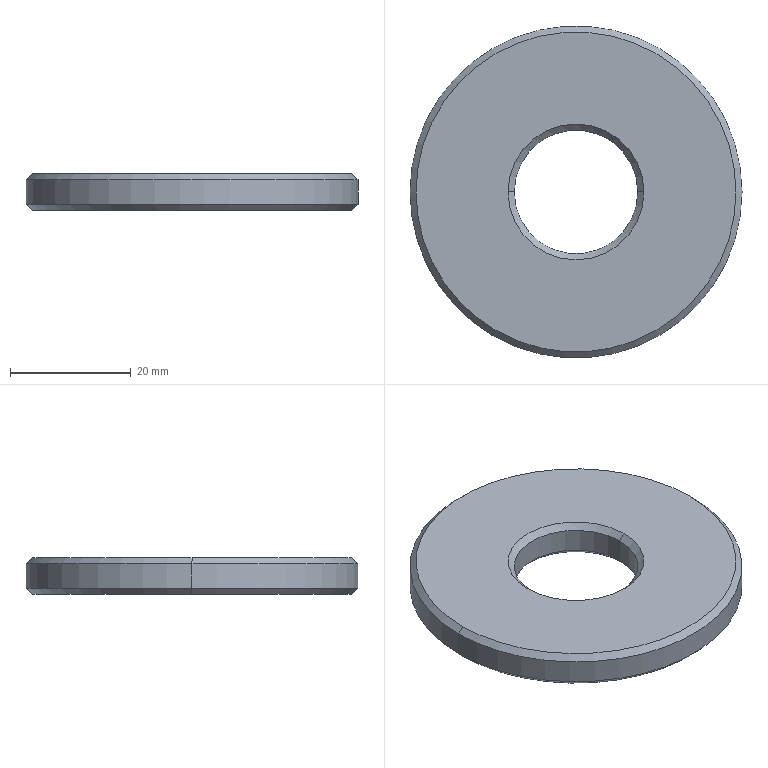Part | STEP file | YCD14007A-08.02.19A Lifting Cylinder Joint Stop Plate Added | 1 solid | 14 faces | box 55 x 55 x 6 mm | volume 12037 mm3 | cone 8 | cylinder 4 | plane 2 | commonest cylinder face diameters 20.5 x2 55 x2
STEP:
#1=CARTESIAN_POINT('',(0.,0.,0.));
#2=DIRECTION('',(0.,0.,1.));
#3=DIRECTION('',(1.,0.,0.));
#4=AXIS2_PLACEMENT_3D('',#1,#2,#3);
#5=CARTESIAN_POINT('',(-26.5,0.,-3.));
#6=VERTEX_POINT('',#5);
#7=CARTESIAN_POINT('',(26.5,0.,-3.));
#8=VERTEX_POINT('',#7);
#9=CARTESIAN_POINT('',(0.,0.,-3.));
#10=DIRECTION('',(0.,0.,-1.));
#11=DIRECTION('',(-1.,0.,0.));
#12=AXIS2_PLACEMENT_3D('',#9,#10,#11);
#13=CIRCLE('',#12,26.5);
#14=CARTESIAN_POINT('',(0.,0.,-2.));
#15=DIRECTION('',(0.,0.,1.));
#16=DIRECTION('',(1.,0.,0.));
#17=AXIS2_PLACEMENT_3D('',#14,#15,#16);
#18=CONICAL_SURFACE('',#17,27.5,0.7854);
#19=CARTESIAN_POINT('',(3.142,-1.));
#20=DIRECTION('',(-1.,0.));
#21=VECTOR('',#20,1.);
#22=LINE('',#19,#21);
#23=(GEOMETRIC_REPRESENTATION_CONTEXT(2)PARAMETRIC_REPRESENTATION_CONTEXT()REPRESENTATION_CONTEXT('',''));
#24=DEFINITIONAL_REPRESENTATION('',(#22),#23);
#25=PCURVE('',#18,#24);
#26=CARTESIAN_POINT('',(27.5,0.,-3.));
#27=DIRECTION('',(0.,0.,-1.));
#28=DIRECTION('',(-1.,0.,0.));
#29=AXIS2_PLACEMENT_3D('',#26,#27,#28);
#30=PLANE('',#29);
#31=CARTESIAN_POINT('',(27.5,0.));
#32=DIRECTION('',(1.,0.));
#33=AXIS2_PLACEMENT_2D('',#31,#32);
#34=CIRCLE('',#33,26.5);
#35=(GEOMETRIC_REPRESENTATION_CONTEXT(2)PARAMETRIC_REPRESENTATION_CONTEXT()REPRESENTATION_CONTEXT('',''));
#36=DEFINITIONAL_REPRESENTATION('',(#34),#35);
#37=PCURVE('',#30,#36);
#38=SURFACE_CURVE('',#13,(#25,#37),.PCURVE_S1.);
#39=EDGE_CURVE('',#6,#8,#38,.T.);
#40=ORIENTED_EDGE('',*,*,#39,.F.);
#41=CARTESIAN_POINT('',(-27.5,0.,-2.));
#42=VERTEX_POINT('',#41);
#43=CARTESIAN_POINT('',(-27.5,0.,-2.));
#44=DIRECTION('',(-0.7071,0.,0.7071));
#45=VECTOR('',#44,1.);
#46=LINE('',#43,#45);
#47=CARTESIAN_POINT('',(3.142,0.));
#48=DIRECTION('',(0.,1.));
#49=VECTOR('',#48,1.);
#50=LINE('',#47,#49);
#51=(GEOMETRIC_REPRESENTATION_CONTEXT(2)PARAMETRIC_REPRESENTATION_CONTEXT()REPRESENTATION_CONTEXT('',''));
#52=DEFINITIONAL_REPRESENTATION('',(#50),#51);
#53=PCURVE('',#18,#52);
#54=CARTESIAN_POINT('',(0.,0.,-2.));
#55=DIRECTION('',(0.,0.,1.));
#56=DIRECTION('',(1.,0.,0.));
#57=AXIS2_PLACEMENT_3D('',#54,#55,#56);
#58=CONICAL_SURFACE('',#57,27.5,0.7854);
#59=CARTESIAN_POINT('',(3.142,0.));
#60=DIRECTION('',(0.,1.));
#61=VECTOR('',#60,1.);
#62=LINE('',#59,#61);
#63=(GEOMETRIC_REPRESENTATION_CONTEXT(2)PARAMETRIC_REPRESENTATION_CONTEXT()REPRESENTATION_CONTEXT('',''));
#64=DEFINITIONAL_REPRESENTATION('',(#62),#63);
#65=PCURVE('',#58,#64);
#66=SURFACE_CURVE('',#46,(#53,#65),.PCURVE_S1.);
#67=EDGE_CURVE('',#6,#42,#66,.T.);
#68=ORIENTED_EDGE('',*,*,#67,.T.);
#69=CARTESIAN_POINT('',(27.5,0.,-2.));
#70=VERTEX_POINT('',#69);
#71=CARTESIAN_POINT('',(0.,0.,-2.));
#72=DIRECTION('',(0.,0.,1.));
#73=DIRECTION('',(-1.,0.,0.));
#74=AXIS2_PLACEMENT_3D('',#71,#72,#73);
#75=CIRCLE('',#74,27.5);
#76=CARTESIAN_POINT('',(-3.142,0.));
#77=DIRECTION('',(1.,0.));
#78=VECTOR('',#77,1.);
#79=LINE('',#76,#78);
#80=(GEOMETRIC_REPRESENTATION_CONTEXT(2)PARAMETRIC_REPRESENTATION_CONTEXT()REPRESENTATION_CONTEXT('',''));
#81=DEFINITIONAL_REPRESENTATION('',(#79),#80);
#82=PCURVE('',#18,#81);
#83=CARTESIAN_POINT('',(0.,0.,1000.));
#84=DIRECTION('',(0.,0.,1.));
#85=DIRECTION('',(1.,0.,0.));
#86=AXIS2_PLACEMENT_3D('',#83,#84,#85);
#87=CYLINDRICAL_SURFACE('',#86,27.5);
#88=CARTESIAN_POINT('',(-3.142,-1002.));
#89=DIRECTION('',(1.,0.));
#90=VECTOR('',#89,1.);
#91=LINE('',#88,#90);
#92=(GEOMETRIC_REPRESENTATION_CONTEXT(2)PARAMETRIC_REPRESENTATION_CONTEXT()REPRESENTATION_CONTEXT('',''));
#93=DEFINITIONAL_REPRESENTATION('',(#91),#92);
#94=PCURVE('',#87,#93);
#95=SURFACE_CURVE('',#75,(#82,#94),.PCURVE_S1.);
#96=EDGE_CURVE('',#70,#42,#95,.T.);
#97=ORIENTED_EDGE('',*,*,#96,.F.);
#98=CARTESIAN_POINT('',(27.5,0.,-2.));
#99=DIRECTION('',(0.7071,0.,0.7071));
#100=VECTOR('',#99,1.);
#101=LINE('',#98,#100);
#102=CARTESIAN_POINT('',(0.,0.));
#103=DIRECTION('',(0.,1.));
#104=VECTOR('',#103,1.);
#105=LINE('',#102,#104);
#106=(GEOMETRIC_REPRESENTATION_CONTEXT(2)PARAMETRIC_REPRESENTATION_CONTEXT()REPRESENTATION_CONTEXT('',''));
#107=DEFINITIONAL_REPRESENTATION('',(#105),#106);
#108=PCURVE('',#18,#107);
#109=CARTESIAN_POINT('',(6.283,0.));
#110=DIRECTION('',(0.,1.));
#111=VECTOR('',#110,1.);
#112=LINE('',#109,#111);
#113=(GEOMETRIC_REPRESENTATION_CONTEXT(2)PARAMETRIC_REPRESENTATION_CONTEXT()REPRESENTATION_CONTEXT('',''));
#114=DEFINITIONAL_REPRESENTATION('',(#112),#113);
#115=PCURVE('',#58,#114);
#116=SURFACE_CURVE('',#101,(#108,#115),.PCURVE_S1.);
#117=EDGE_CURVE('',#8,#70,#116,.T.);
#118=ORIENTED_EDGE('',*,*,#117,.F.);
#119=EDGE_LOOP('',(#40,#68,#97,#118));
#120=FACE_BOUND('',#119,.T.);
#121=ADVANCED_FACE('',(#120),#18,.T.);
#122=CARTESIAN_POINT('',(26.5,0.,3.));
#123=VERTEX_POINT('',#122);
#124=CARTESIAN_POINT('',(-26.5,0.,3.));
#125=VERTEX_POINT('',#124);
#126=CARTESIAN_POINT('',(0.,0.,3.));
#127=DIRECTION('',(0.,0.,1.));
#128=DIRECTION('',(1.,0.,0.));
#129=AXIS2_PLACEMENT_3D('',#126,#127,#128);
#130=CIRCLE('',#129,26.5);
#131=CARTESIAN_POINT('',(0.,0.,3.));
#132=DIRECTION('',(0.,0.,-1.));
#133=DIRECTION('',(-1.,0.,0.));
#134=AXIS2_PLACEMENT_3D('',#131,#132,#133);
#135=CONICAL_SURFACE('',#134,26.5,0.7854);
#136=CARTESIAN_POINT('',(3.142,0.));
#137=DIRECTION('',(-1.,0.));
#138=VECTOR('',#137,1.);
#139=LINE('',#136,#138);
#140=(GEOMETRIC_REPRESENTATION_CONTEXT(2)PARAMETRIC_REPRESENTATION_CONTEXT()REPRESENTATION_CONTEXT('',''));
#141=DEFINITIONAL_REPRESENTATION('',(#139),#140);
#142=PCURVE('',#135,#141);
#143=CARTESIAN_POINT('',(10.25,0.,3.));
#144=DIRECTION('',(0.,0.,1.));
#145=DIRECTION('',(1.,0.,0.));
#146=AXIS2_PLACEMENT_3D('',#143,#144,#145);
#147=PLANE('',#146);
#148=CARTESIAN_POINT('',(-10.25,0.));
#149=DIRECTION('',(1.,0.));
#150=AXIS2_PLACEMENT_2D('',#148,#149);
#151=CIRCLE('',#150,26.5);
#152=(GEOMETRIC_REPRESENTATION_CONTEXT(2)PARAMETRIC_REPRESENTATION_CONTEXT()REPRESENTATION_CONTEXT('',''));
#153=DEFINITIONAL_REPRESENTATION('',(#151),#152);
#154=PCURVE('',#147,#153);
#155=SURFACE_CURVE('',#130,(#142,#154),.PCURVE_S1.);
#156=EDGE_CURVE('',#123,#125,#155,.T.);
#157=ORIENTED_EDGE('',*,*,#156,.F.);
#158=CARTESIAN_POINT('',(27.5,0.,2.));
#159=VERTEX_POINT('',#158);
#160=CARTESIAN_POINT('',(26.5,0.,3.));
#161=DIRECTION('',(0.7071,0.,-0.7071));
#162=VECTOR('',#161,1.);
#163=LINE('',#160,#162);
#164=CARTESIAN_POINT('',(3.142,0.));
#165=DIRECTION('',(0.,1.));
#166=VECTOR('',#165,1.);
#167=LINE('',#164,#166);
#168=(GEOMETRIC_REPRESENTATION_CONTEXT(2)PARAMETRIC_REPRESENTATION_CONTEXT()REPRESENTATION_CONTEXT('',''));
#169=DEFINITIONAL_REPRESENTATION('',(#167),#168);
#170=PCURVE('',#135,#169);
#171=CARTESIAN_POINT('',(0.,0.,3.));
#172=DIRECTION('',(0.,0.,-1.));
#173=DIRECTION('',(-1.,0.,0.));
#174=AXIS2_PLACEMENT_3D('',#171,#172,#173);
#175=CONICAL_SURFACE('',#174,26.5,0.7854);
#176=CARTESIAN_POINT('',(3.142,0.));
#177=DIRECTION('',(0.,1.));
#178=VECTOR('',#177,1.);
#179=LINE('',#176,#178);
#180=(GEOMETRIC_REPRESENTATION_CONTEXT(2)PARAMETRIC_REPRESENTATION_CONTEXT()REPRESENTATION_CONTEXT('',''));
#181=DEFINITIONAL_REPRESENTATION('',(#179),#180);
#182=PCURVE('',#175,#181);
#183=SURFACE_CURVE('',#163,(#170,#182),.PCURVE_S1.);
#184=EDGE_CURVE('',#123,#159,#183,.T.);
#185=ORIENTED_EDGE('',*,*,#184,.T.);
#186=CARTESIAN_POINT('',(-27.5,0.,2.));
#187=VERTEX_POINT('',#186);
#188=CARTESIAN_POINT('',(0.,0.,2.));
#189=DIRECTION('',(0.,0.,-1.));
#190=DIRECTION('',(1.,0.,0.));
#191=AXIS2_PLACEMENT_3D('',#188,#189,#190);
#192=CIRCLE('',#191,27.5);
#193=CARTESIAN_POINT('',(-3.142,1.));
#194=DIRECTION('',(1.,0.));
#195=VECTOR('',#194,1.);
#196=LINE('',#193,#195);
#197=(GEOMETRIC_REPRESENTATION_CONTEXT(2)PARAMETRIC_REPRESENTATION_CONTEXT()REPRESENTATION_CONTEXT('',''));
#198=DEFINITIONAL_REPRESENTATION('',(#196),#197);
#199=PCURVE('',#135,#198);
#200=CARTESIAN_POINT('',(6.283,-998.));
#201=DIRECTION('',(-1.,0.));
#202=VECTOR('',#201,1.);
#203=LINE('',#200,#202);
#204=(GEOMETRIC_REPRESENTATION_CONTEXT(2)PARAMETRIC_REPRESENTATION_CONTEXT()REPRESENTATION_CONTEXT('',''));
#205=DEFINITIONAL_REPRESENTATION('',(#203),#204);
#206=PCURVE('',#87,#205);
#207=SURFACE_CURVE('',#192,(#199,#206),.PCURVE_S1.);
#208=EDGE_CURVE('',#187,#159,#207,.T.);
#209=ORIENTED_EDGE('',*,*,#208,.F.);
#210=CARTESIAN_POINT('',(-26.5,0.,3.));
#211=DIRECTION('',(-0.7071,0.,-0.7071));
#212=VECTOR('',#211,1.);
#213=LINE('',#210,#212);
#214=CARTESIAN_POINT('',(0.,0.));
#215=DIRECTION('',(0.,1.));
#216=VECTOR('',#215,1.);
#217=LINE('',#214,#216);
#218=(GEOMETRIC_REPRESENTATION_CONTEXT(2)PARAMETRIC_REPRESENTATION_CONTEXT()REPRESENTATION_CONTEXT('',''));
#219=DEFINITIONAL_REPRESENTATION('',(#217),#218);
#220=PCURVE('',#135,#219);
#221=CARTESIAN_POINT('',(6.283,0.));
#222=DIRECTION('',(0.,1.));
#223=VECTOR('',#222,1.);
#224=LINE('',#221,#223);
#225=(GEOMETRIC_REPRESENTATION_CONTEXT(2)PARAMETRIC_REPRESENTATION_CONTEXT()REPRESENTATION_CONTEXT('',''));
#226=DEFINITIONAL_REPRESENTATION('',(#224),#225);
#227=PCURVE('',#175,#226);
#228=SURFACE_CURVE('',#213,(#220,#227),.PCURVE_S1.);
#229=EDGE_CURVE('',#125,#187,#228,.T.);
#230=ORIENTED_EDGE('',*,*,#229,.F.);
#231=EDGE_LOOP('',(#157,#185,#209,#230));
#232=FACE_BOUND('',#231,.T.);
#233=ADVANCED_FACE('',(#232),#135,.T.);
#234=CARTESIAN_POINT('',(-10.25,0.,-2.));
#235=VERTEX_POINT('',#234);
#236=CARTESIAN_POINT('',(-11.25,0.,-3.));
#237=VERTEX_POINT('',#236);
#238=CARTESIAN_POINT('',(-11.25,0.,-3.));
#239=DIRECTION('',(-0.7071,0.,-0.7071));
#240=VECTOR('',#239,1.);
#241=LINE('',#238,#240);
#242=CARTESIAN_POINT('',(0.,0.,-3.));
#243=DIRECTION('',(0.,0.,-1.));
#244=DIRECTION('',(-1.,0.,0.));
#245=AXIS2_PLACEMENT_3D('',#242,#243,#244);
#246=CONICAL_SURFACE('',#245,11.25,0.7854);
#247=CARTESIAN_POINT('',(6.283,0.));
#248=DIRECTION('',(0.,1.));
#249=VECTOR('',#248,1.);
#250=LINE('',#247,#249);
#251=(GEOMETRIC_REPRESENTATION_CONTEXT(2)PARAMETRIC_REPRESENTATION_CONTEXT()REPRESENTATION_CONTEXT('',''));
#252=DEFINITIONAL_REPRESENTATION('',(#250),#251);
#253=PCURVE('',#246,#252);
#254=CARTESIAN_POINT('',(0.,0.,-3.));
#255=DIRECTION('',(0.,0.,-1.));
#256=DIRECTION('',(-1.,0.,0.));
#257=AXIS2_PLACEMENT_3D('',#254,#255,#256);
#258=CONICAL_SURFACE('',#257,11.25,0.7854);
#259=CARTESIAN_POINT('',(0.,0.));
#260=DIRECTION('',(0.,1.));
#261=VECTOR('',#260,1.);
#262=LINE('',#259,#261);
#263=(GEOMETRIC_REPRESENTATION_CONTEXT(2)PARAMETRIC_REPRESENTATION_CONTEXT()REPRESENTATION_CONTEXT('',''));
#264=DEFINITIONAL_REPRESENTATION('',(#262),#263);
#265=PCURVE('',#258,#264);
#266=SURFACE_CURVE('',#241,(#253,#265),.PCURVE_S1.);
#267=EDGE_CURVE('',#235,#237,#266,.T.);
#268=ORIENTED_EDGE('',*,*,#267,.T.);
#269=CARTESIAN_POINT('',(11.25,0.,-3.));
#270=VERTEX_POINT('',#269);
#271=CARTESIAN_POINT('',(0.,0.,-3.));
#272=DIRECTION('',(0.,0.,1.));
#273=DIRECTION('',(-1.,0.,0.));
#274=AXIS2_PLACEMENT_3D('',#271,#272,#273);
#275=CIRCLE('',#274,11.25);
#276=CARTESIAN_POINT('',(6.283,0.));
#277=DIRECTION('',(-1.,0.));
#278=VECTOR('',#277,1.);
#279=LINE('',#276,#278);
#280=(GEOMETRIC_REPRESENTATION_CONTEXT(2)PARAMETRIC_REPRESENTATION_CONTEXT()REPRESENTATION_CONTEXT('',''));
#281=DEFINITIONAL_REPRESENTATION('',(#279),#280);
#282=PCURVE('',#246,#281);
#283=CARTESIAN_POINT('',(38.75,0.));
#284=CARTESIAN_POINT('',(38.75,-19.486));
#285=CARTESIAN_POINT('',(21.875,-9.743));
#286=CARTESIAN_POINT('',(5.,0.));
#287=CARTESIAN_POINT('',(21.875,9.743));
#288=CARTESIAN_POINT('',(38.75,19.486));
#289=CARTESIAN_POINT('',(38.75,0.));
#290=(BOUNDED_CURVE()B_SPLINE_CURVE(2,(#283,#284,#285,#286,#287,#288,#289),.UNSPECIFIED.,.T.,.F.)B_SPLINE_CURVE_WITH_KNOTS((1,2,2,2,2,1),(-2.094,0.,2.094,4.189,6.283,8.378),.UNSPECIFIED.)CURVE()GEOMETRIC_REPRESENTATION_ITEM()RATIONAL_B_SPLINE_CURVE((1.,0.5,1.,0.5,1.,0.5,1.))REPRESENTATION_ITEM(''));
#291=(GEOMETRIC_REPRESENTATION_CONTEXT(2)PARAMETRIC_REPRESENTATION_CONTEXT()REPRESENTATION_CONTEXT('',''));
#292=DEFINITIONAL_REPRESENTATION('',(#290),#291);
#293=PCURVE('',#30,#292);
#294=SURFACE_CURVE('',#275,(#282,#293),.PCURVE_S1.);
#295=EDGE_CURVE('',#237,#270,#294,.T.);
#296=ORIENTED_EDGE('',*,*,#295,.T.);
#297=CARTESIAN_POINT('',(10.25,0.,-2.));
#298=VERTEX_POINT('',#297);
#299=CARTESIAN_POINT('',(11.25,0.,-3.));
#300=DIRECTION('',(0.7071,0.,-0.7071));
#301=VECTOR('',#300,1.);
#302=LINE('',#299,#301);
#303=CARTESIAN_POINT('',(3.142,0.));
#304=DIRECTION('',(0.,1.));
#305=VECTOR('',#304,1.);
#306=LINE('',#303,#305);
#307=(GEOMETRIC_REPRESENTATION_CONTEXT(2)PARAMETRIC_REPRESENTATION_CONTEXT()REPRESENTATION_CONTEXT('',''));
#308=DEFINITIONAL_REPRESENTATION('',(#306),#307);
#309=PCURVE('',#246,#308);
#310=CARTESIAN_POINT('',(3.142,0.));
#311=DIRECTION('',(0.,1.));
#312=VECTOR('',#311,1.);
#313=LINE('',#310,#312);
#314=(GEOMETRIC_REPRESENTATION_CONTEXT(2)PARAMETRIC_REPRESENTATION_CONTEXT()REPRESENTATION_CONTEXT('',''));
#315=DEFINITIONAL_REPRESENTATION('',(#313),#314);
#316=PCURVE('',#258,#315);
#317=SURFACE_CURVE('',#302,(#309,#316),.PCURVE_S1.);
#318=EDGE_CURVE('',#298,#270,#317,.T.);
#319=ORIENTED_EDGE('',*,*,#318,.F.);
#320=CARTESIAN_POINT('',(0.,0.,-2.));
#321=DIRECTION('',(0.,0.,-1.));
#322=DIRECTION('',(-1.,0.,0.));
#323=AXIS2_PLACEMENT_3D('',#320,#321,#322);
#324=CIRCLE('',#323,10.25);
#325=CARTESIAN_POINT('',(0.,-1.));
#326=DIRECTION('',(1.,0.));
#327=VECTOR('',#326,1.);
#328=LINE('',#325,#327);
#329=(GEOMETRIC_REPRESENTATION_CONTEXT(2)PARAMETRIC_REPRESENTATION_CONTEXT()REPRESENTATION_CONTEXT('',''));
#330=DEFINITIONAL_REPRESENTATION('',(#328),#329);
#331=PCURVE('',#246,#330);
#332=CARTESIAN_POINT('',(0.,0.,1000.));
#333=DIRECTION('',(0.,0.,1.));
#334=DIRECTION('',(1.,0.,0.));
#335=AXIS2_PLACEMENT_3D('',#332,#333,#334);
#336=CYLINDRICAL_SURFACE('',#335,10.25);
#337=CARTESIAN_POINT('',(9.425,-1002.));
#338=DIRECTION('',(-1.,0.));
#339=VECTOR('',#338,1.);
#340=LINE('',#337,#339);
#341=(GEOMETRIC_REPRESENTATION_CONTEXT(2)PARAMETRIC_REPRESENTATION_CONTEXT()REPRESENTATION_CONTEXT('',''));
#342=DEFINITIONAL_REPRESENTATION('',(#340),#341);
#343=PCURVE('',#336,#342);
#344=SURFACE_CURVE('',#324,(#331,#343),.PCURVE_S1.);
#345=EDGE_CURVE('',#298,#235,#344,.T.);
#346=ORIENTED_EDGE('',*,*,#345,.T.);
#347=EDGE_LOOP('',(#268,#296,#319,#346));
#348=FACE_BOUND('',#347,.F.);
#349=ADVANCED_FACE('',(#348),#246,.F.);
#350=CARTESIAN_POINT('',(10.25,0.,2.));
#351=VERTEX_POINT('',#350);
#352=CARTESIAN_POINT('',(11.25,0.,3.));
#353=VERTEX_POINT('',#352);
#354=CARTESIAN_POINT('',(10.25,0.,2.));
#355=DIRECTION('',(0.7071,0.,0.7071));
#356=VECTOR('',#355,1.);
#357=LINE('',#354,#356);
#358=CARTESIAN_POINT('',(0.,0.,2.));
#359=DIRECTION('',(0.,0.,1.));
#360=DIRECTION('',(1.,0.,0.));
#361=AXIS2_PLACEMENT_3D('',#358,#359,#360);
#362=CONICAL_SURFACE('',#361,10.25,0.7854);
#363=CARTESIAN_POINT('',(6.283,0.));
#364=DIRECTION('',(0.,1.));
#365=VECTOR('',#364,1.);
#366=LINE('',#363,#365);
#367=(GEOMETRIC_REPRESENTATION_CONTEXT(2)PARAMETRIC_REPRESENTATION_CONTEXT()REPRESENTATION_CONTEXT('',''));
#368=DEFINITIONAL_REPRESENTATION('',(#366),#367);
#369=PCURVE('',#362,#368);
#370=CARTESIAN_POINT('',(0.,0.,2.));
#371=DIRECTION('',(0.,0.,1.));
#372=DIRECTION('',(1.,0.,0.));
#373=AXIS2_PLACEMENT_3D('',#370,#371,#372);
#374=CONICAL_SURFACE('',#373,10.25,0.7854);
#375=CARTESIAN_POINT('',(0.,0.));
#376=DIRECTION('',(0.,1.));
#377=VECTOR('',#376,1.);
#378=LINE('',#375,#377);
#379=(GEOMETRIC_REPRESENTATION_CONTEXT(2)PARAMETRIC_REPRESENTATION_CONTEXT()REPRESENTATION_CONTEXT('',''));
#380=DEFINITIONAL_REPRESENTATION('',(#378),#379);
#381=PCURVE('',#374,#380);
#382=SURFACE_CURVE('',#357,(#369,#381),.PCURVE_S1.);
#383=EDGE_CURVE('',#351,#353,#382,.T.);
#384=ORIENTED_EDGE('',*,*,#383,.T.);
#385=CARTESIAN_POINT('',(-11.25,0.,3.));
#386=VERTEX_POINT('',#385);
#387=CARTESIAN_POINT('',(0.,0.,3.));
#388=DIRECTION('',(0.,0.,-1.));
#389=DIRECTION('',(1.,0.,0.));
#390=AXIS2_PLACEMENT_3D('',#387,#388,#389);
#391=CIRCLE('',#390,11.25);
#392=CARTESIAN_POINT('',(6.283,1.));
#393=DIRECTION('',(-1.,0.));
#394=VECTOR('',#393,1.);
#395=LINE('',#392,#394);
#396=(GEOMETRIC_REPRESENTATION_CONTEXT(2)PARAMETRIC_REPRESENTATION_CONTEXT()REPRESENTATION_CONTEXT('',''));
#397=DEFINITIONAL_REPRESENTATION('',(#395),#396);
#398=PCURVE('',#362,#397);
#399=CARTESIAN_POINT('',(1.,0.));
#400=CARTESIAN_POINT('',(1.,-19.486));
#401=CARTESIAN_POINT('',(-15.875,-9.743));
#402=CARTESIAN_POINT('',(-32.75,0.));
#403=CARTESIAN_POINT('',(-15.875,9.743));
#404=CARTESIAN_POINT('',(1.,19.486));
#405=CARTESIAN_POINT('',(1.,0.));
#406=(BOUNDED_CURVE()B_SPLINE_CURVE(2,(#399,#400,#401,#402,#403,#404,#405),.UNSPECIFIED.,.T.,.F.)B_SPLINE_CURVE_WITH_KNOTS((1,2,2,2,2,1),(-2.094,0.,2.094,4.189,6.283,8.378),.UNSPECIFIED.)CURVE()GEOMETRIC_REPRESENTATION_ITEM()RATIONAL_B_SPLINE_CURVE((1.,0.5,1.,0.5,1.,0.5,1.))REPRESENTATION_ITEM(''));
#407=(GEOMETRIC_REPRESENTATION_CONTEXT(2)PARAMETRIC_REPRESENTATION_CONTEXT()REPRESENTATION_CONTEXT('',''));
#408=DEFINITIONAL_REPRESENTATION('',(#406),#407);
#409=PCURVE('',#147,#408);
#410=SURFACE_CURVE('',#391,(#398,#409),.PCURVE_S1.);
#411=EDGE_CURVE('',#353,#386,#410,.T.);
#412=ORIENTED_EDGE('',*,*,#411,.T.);
#413=CARTESIAN_POINT('',(-10.25,0.,2.));
#414=VERTEX_POINT('',#413);
#415=CARTESIAN_POINT('',(-10.25,0.,2.));
#416=DIRECTION('',(-0.7071,0.,0.7071));
#417=VECTOR('',#416,1.);
#418=LINE('',#415,#417);
#419=CARTESIAN_POINT('',(3.142,0.));
#420=DIRECTION('',(0.,1.));
#421=VECTOR('',#420,1.);
#422=LINE('',#419,#421);
#423=(GEOMETRIC_REPRESENTATION_CONTEXT(2)PARAMETRIC_REPRESENTATION_CONTEXT()REPRESENTATION_CONTEXT('',''));
#424=DEFINITIONAL_REPRESENTATION('',(#422),#423);
#425=PCURVE('',#362,#424);
#426=CARTESIAN_POINT('',(3.142,0.));
#427=DIRECTION('',(0.,1.));
#428=VECTOR('',#427,1.);
#429=LINE('',#426,#428);
#430=(GEOMETRIC_REPRESENTATION_CONTEXT(2)PARAMETRIC_REPRESENTATION_CONTEXT()REPRESENTATION_CONTEXT('',''));
#431=DEFINITIONAL_REPRESENTATION('',(#429),#430);
#432=PCURVE('',#374,#431);
#433=SURFACE_CURVE('',#418,(#425,#432),.PCURVE_S1.);
#434=EDGE_CURVE('',#414,#386,#433,.T.);
#435=ORIENTED_EDGE('',*,*,#434,.F.);
#436=CARTESIAN_POINT('',(0.,0.,2.));
#437=DIRECTION('',(0.,0.,1.));
#438=DIRECTION('',(1.,0.,0.));
#439=AXIS2_PLACEMENT_3D('',#436,#437,#438);
#440=CIRCLE('',#439,10.25);
#441=CARTESIAN_POINT('',(0.,0.));
#442=DIRECTION('',(1.,0.));
#443=VECTOR('',#442,1.);
#444=LINE('',#441,#443);
#445=(GEOMETRIC_REPRESENTATION_CONTEXT(2)PARAMETRIC_REPRESENTATION_CONTEXT()REPRESENTATION_CONTEXT('',''));
#446=DEFINITIONAL_REPRESENTATION('',(#444),#445);
#447=PCURVE('',#362,#446);
#448=CARTESIAN_POINT('',(0.,-998.));
#449=DIRECTION('',(1.,0.));
#450=VECTOR('',#449,1.);
#451=LINE('',#448,#450);
#452=(GEOMETRIC_REPRESENTATION_CONTEXT(2)PARAMETRIC_REPRESENTATION_CONTEXT()REPRESENTATION_CONTEXT('',''));
#453=DEFINITIONAL_REPRESENTATION('',(#451),#452);
#454=PCURVE('',#336,#453);
#455=SURFACE_CURVE('',#440,(#447,#454),.PCURVE_S1.);
#456=EDGE_CURVE('',#414,#351,#455,.T.);
#457=ORIENTED_EDGE('',*,*,#456,.T.);
#458=EDGE_LOOP('',(#384,#412,#435,#457));
#459=FACE_BOUND('',#458,.F.);
#460=ADVANCED_FACE('',(#459),#362,.F.);
#461=CARTESIAN_POINT('',(10.25,0.,1000.));
#462=DIRECTION('',(0.,0.,1.));
#463=VECTOR('',#462,1.);
#464=LINE('',#461,#463);
#465=CARTESIAN_POINT('',(6.283,0.));
#466=DIRECTION('',(0.,1.));
#467=VECTOR('',#466,1.);
#468=LINE('',#465,#467);
#469=(GEOMETRIC_REPRESENTATION_CONTEXT(2)PARAMETRIC_REPRESENTATION_CONTEXT()REPRESENTATION_CONTEXT('',''));
#470=DEFINITIONAL_REPRESENTATION('',(#468),#469);
#471=PCURVE('',#336,#470);
#472=CARTESIAN_POINT('',(0.,0.,1000.));
#473=DIRECTION('',(0.,0.,1.));
#474=DIRECTION('',(1.,0.,0.));
#475=AXIS2_PLACEMENT_3D('',#472,#473,#474);
#476=CYLINDRICAL_SURFACE('',#475,10.25);
#477=CARTESIAN_POINT('',(0.,0.));
#478=DIRECTION('',(0.,1.));
#479=VECTOR('',#478,1.);
#480=LINE('',#477,#479);
#481=(GEOMETRIC_REPRESENTATION_CONTEXT(2)PARAMETRIC_REPRESENTATION_CONTEXT()REPRESENTATION_CONTEXT('',''));
#482=DEFINITIONAL_REPRESENTATION('',(#480),#481);
#483=PCURVE('',#476,#482);
#484=SURFACE_CURVE('',#464,(#471,#483),.PCURVE_S1.);
#485=EDGE_CURVE('',#298,#351,#484,.T.);
#486=ORIENTED_EDGE('',*,*,#485,.T.);
#487=ORIENTED_EDGE('',*,*,#456,.F.);
#488=CARTESIAN_POINT('',(-10.25,0.,1000.));
#489=DIRECTION('',(0.,0.,1.));
#490=VECTOR('',#489,1.);
#491=LINE('',#488,#490);
#492=CARTESIAN_POINT('',(3.142,0.));
#493=DIRECTION('',(0.,1.));
#494=VECTOR('',#493,1.);
#495=LINE('',#492,#494);
#496=(GEOMETRIC_REPRESENTATION_CONTEXT(2)PARAMETRIC_REPRESENTATION_CONTEXT()REPRESENTATION_CONTEXT('',''));
#497=DEFINITIONAL_REPRESENTATION('',(#495),#496);
#498=PCURVE('',#336,#497);
#499=CARTESIAN_POINT('',(3.142,0.));
#500=DIRECTION('',(0.,1.));
#501=VECTOR('',#500,1.);
#502=LINE('',#499,#501);
#503=(GEOMETRIC_REPRESENTATION_CONTEXT(2)PARAMETRIC_REPRESENTATION_CONTEXT()REPRESENTATION_CONTEXT('',''));
#504=DEFINITIONAL_REPRESENTATION('',(#502),#503);
#505=PCURVE('',#476,#504);
#506=SURFACE_CURVE('',#491,(#498,#505),.PCURVE_S1.);
#507=EDGE_CURVE('',#235,#414,#506,.T.);
#508=ORIENTED_EDGE('',*,*,#507,.F.);
#509=ORIENTED_EDGE('',*,*,#345,.F.);
#510=EDGE_LOOP('',(#486,#487,#508,#509));
#511=FACE_BOUND('',#510,.F.);
#512=ADVANCED_FACE('',(#511),#336,.F.);
#513=ORIENTED_EDGE('',*,*,#96,.T.);
#514=CARTESIAN_POINT('',(-27.5,0.,1000.));
#515=DIRECTION('',(0.,0.,1.));
#516=VECTOR('',#515,1.);
#517=LINE('',#514,#516);
#518=CARTESIAN_POINT('',(3.142,0.));
#519=DIRECTION('',(0.,1.));
#520=VECTOR('',#519,1.);
#521=LINE('',#518,#520);
#522=(GEOMETRIC_REPRESENTATION_CONTEXT(2)PARAMETRIC_REPRESENTATION_CONTEXT()REPRESENTATION_CONTEXT('',''));
#523=DEFINITIONAL_REPRESENTATION('',(#521),#522);
#524=PCURVE('',#87,#523);
#525=CARTESIAN_POINT('',(0.,0.,1000.));
#526=DIRECTION('',(0.,0.,1.));
#527=DIRECTION('',(1.,0.,0.));
#528=AXIS2_PLACEMENT_3D('',#525,#526,#527);
#529=CYLINDRICAL_SURFACE('',#528,27.5);
#530=CARTESIAN_POINT('',(3.142,0.));
#531=DIRECTION('',(0.,1.));
#532=VECTOR('',#531,1.);
#533=LINE('',#530,#532);
#534=(GEOMETRIC_REPRESENTATION_CONTEXT(2)PARAMETRIC_REPRESENTATION_CONTEXT()REPRESENTATION_CONTEXT('',''));
#535=DEFINITIONAL_REPRESENTATION('',(#533),#534);
#536=PCURVE('',#529,#535);
#537=SURFACE_CURVE('',#517,(#524,#536),.PCURVE_S1.);
#538=EDGE_CURVE('',#42,#187,#537,.T.);
#539=ORIENTED_EDGE('',*,*,#538,.T.);
#540=ORIENTED_EDGE('',*,*,#208,.T.);
#541=CARTESIAN_POINT('',(27.5,0.,1000.));
#542=DIRECTION('',(0.,0.,1.));
#543=VECTOR('',#542,1.);
#544=LINE('',#541,#543);
#545=CARTESIAN_POINT('',(0.,0.));
#546=DIRECTION('',(0.,1.));
#547=VECTOR('',#546,1.);
#548=LINE('',#545,#547);
#549=(GEOMETRIC_REPRESENTATION_CONTEXT(2)PARAMETRIC_REPRESENTATION_CONTEXT()REPRESENTATION_CONTEXT('',''));
#550=DEFINITIONAL_REPRESENTATION('',(#548),#549);
#551=PCURVE('',#87,#550);
#552=CARTESIAN_POINT('',(6.283,0.));
#553=DIRECTION('',(0.,1.));
#554=VECTOR('',#553,1.);
#555=LINE('',#552,#554);
#556=(GEOMETRIC_REPRESENTATION_CONTEXT(2)PARAMETRIC_REPRESENTATION_CONTEXT()REPRESENTATION_CONTEXT('',''));
#557=DEFINITIONAL_REPRESENTATION('',(#555),#556);
#558=PCURVE('',#529,#557);
#559=SURFACE_CURVE('',#544,(#551,#558),.PCURVE_S1.);
#560=EDGE_CURVE('',#70,#159,#559,.T.);
#561=ORIENTED_EDGE('',*,*,#560,.F.);
#562=EDGE_LOOP('',(#513,#539,#540,#561));
#563=FACE_BOUND('',#562,.T.);
#564=ADVANCED_FACE('',(#563),#87,.T.);
#565=ORIENTED_EDGE('',*,*,#538,.F.);
#566=CARTESIAN_POINT('',(0.,0.,-2.));
#567=DIRECTION('',(0.,0.,1.));
#568=DIRECTION('',(-1.,0.,0.));
#569=AXIS2_PLACEMENT_3D('',#566,#567,#568);
#570=CIRCLE('',#569,27.5);
#571=CARTESIAN_POINT('',(3.142,-1002.));
#572=DIRECTION('',(1.,0.));
#573=VECTOR('',#572,1.);
#574=LINE('',#571,#573);
#575=(GEOMETRIC_REPRESENTATION_CONTEXT(2)PARAMETRIC_REPRESENTATION_CONTEXT()REPRESENTATION_CONTEXT('',''));
#576=DEFINITIONAL_REPRESENTATION('',(#574),#575);
#577=PCURVE('',#529,#576);
#578=CARTESIAN_POINT('',(3.142,0.));
#579=DIRECTION('',(1.,0.));
#580=VECTOR('',#579,1.);
#581=LINE('',#578,#580);
#582=(GEOMETRIC_REPRESENTATION_CONTEXT(2)PARAMETRIC_REPRESENTATION_CONTEXT()REPRESENTATION_CONTEXT('',''));
#583=DEFINITIONAL_REPRESENTATION('',(#581),#582);
#584=PCURVE('',#58,#583);
#585=SURFACE_CURVE('',#570,(#577,#584),.PCURVE_S1.);
#586=EDGE_CURVE('',#42,#70,#585,.T.);
#587=ORIENTED_EDGE('',*,*,#586,.T.);
#588=ORIENTED_EDGE('',*,*,#560,.T.);
#589=CARTESIAN_POINT('',(0.,0.,2.));
#590=DIRECTION('',(0.,0.,-1.));
#591=DIRECTION('',(1.,0.,0.));
#592=AXIS2_PLACEMENT_3D('',#589,#590,#591);
#593=CIRCLE('',#592,27.5);
#594=CARTESIAN_POINT('',(6.283,-998.));
#595=DIRECTION('',(-1.,0.));
#596=VECTOR('',#595,1.);
#597=LINE('',#594,#596);
#598=(GEOMETRIC_REPRESENTATION_CONTEXT(2)PARAMETRIC_REPRESENTATION_CONTEXT()REPRESENTATION_CONTEXT('',''));
#599=DEFINITIONAL_REPRESENTATION('',(#597),#598);
#600=PCURVE('',#529,#599);
#601=CARTESIAN_POINT('',(3.142,1.));
#602=DIRECTION('',(1.,0.));
#603=VECTOR('',#602,1.);
#604=LINE('',#601,#603);
#605=(GEOMETRIC_REPRESENTATION_CONTEXT(2)PARAMETRIC_REPRESENTATION_CONTEXT()REPRESENTATION_CONTEXT('',''));
#606=DEFINITIONAL_REPRESENTATION('',(#604),#605);
#607=PCURVE('',#175,#606);
#608=SURFACE_CURVE('',#593,(#600,#607),.PCURVE_S1.);
#609=EDGE_CURVE('',#159,#187,#608,.T.);
#610=ORIENTED_EDGE('',*,*,#609,.T.);
#611=EDGE_LOOP('',(#565,#587,#588,#610));
#612=FACE_BOUND('',#611,.T.);
#613=ADVANCED_FACE('',(#612),#529,.T.);
#614=ORIENTED_EDGE('',*,*,#295,.T.);
#615=CARTESIAN_POINT('',(0.,0.,-3.));
#616=DIRECTION('',(0.,0.,1.));
#617=DIRECTION('',(-1.,0.,0.));
#618=AXIS2_PLACEMENT_3D('',#615,#616,#617);
#619=CIRCLE('',#618,11.25);
#620=CARTESIAN_POINT('',(38.75,0.));
#621=CARTESIAN_POINT('',(38.75,-19.486));
#622=CARTESIAN_POINT('',(21.875,-9.743));
#623=CARTESIAN_POINT('',(5.,0.));
#624=CARTESIAN_POINT('',(21.875,9.743));
#625=CARTESIAN_POINT('',(38.75,19.486));
#626=CARTESIAN_POINT('',(38.75,0.));
#627=(BOUNDED_CURVE()B_SPLINE_CURVE(2,(#620,#621,#622,#623,#624,#625,#626),.UNSPECIFIED.,.T.,.F.)B_SPLINE_CURVE_WITH_KNOTS((1,2,2,2,2,1),(-2.094,0.,2.094,4.189,6.283,8.378),.UNSPECIFIED.)CURVE()GEOMETRIC_REPRESENTATION_ITEM()RATIONAL_B_SPLINE_CURVE((1.,0.5,1.,0.5,1.,0.5,1.))REPRESENTATION_ITEM(''));
#628=(GEOMETRIC_REPRESENTATION_CONTEXT(2)PARAMETRIC_REPRESENTATION_CONTEXT()REPRESENTATION_CONTEXT('',''));
#629=DEFINITIONAL_REPRESENTATION('',(#627),#628);
#630=PCURVE('',#30,#629);
#631=CARTESIAN_POINT('',(6.283,0.));
#632=DIRECTION('',(-1.,0.));
#633=VECTOR('',#632,1.);
#634=LINE('',#631,#633);
#635=(GEOMETRIC_REPRESENTATION_CONTEXT(2)PARAMETRIC_REPRESENTATION_CONTEXT()REPRESENTATION_CONTEXT('',''));
#636=DEFINITIONAL_REPRESENTATION('',(#634),#635);
#637=PCURVE('',#258,#636);
#638=SURFACE_CURVE('',#619,(#630,#637),.PCURVE_S1.);
#639=EDGE_CURVE('',#270,#237,#638,.T.);
#640=ORIENTED_EDGE('',*,*,#639,.T.);
#641=EDGE_LOOP('',(#614,#640));
#642=FACE_BOUND('',#641,.T.);
#643=CARTESIAN_POINT('',(0.,0.,-3.));
#644=DIRECTION('',(0.,0.,-1.));
#645=DIRECTION('',(-1.,0.,0.));
#646=AXIS2_PLACEMENT_3D('',#643,#644,#645);
#647=CIRCLE('',#646,26.5);
#648=CARTESIAN_POINT('',(27.5,0.));
#649=DIRECTION('',(1.,0.));
#650=AXIS2_PLACEMENT_2D('',#648,#649);
#651=CIRCLE('',#650,26.5);
#652=(GEOMETRIC_REPRESENTATION_CONTEXT(2)PARAMETRIC_REPRESENTATION_CONTEXT()REPRESENTATION_CONTEXT('',''));
#653=DEFINITIONAL_REPRESENTATION('',(#651),#652);
#654=PCURVE('',#30,#653);
#655=CARTESIAN_POINT('',(9.425,-1.));
#656=DIRECTION('',(-1.,0.));
#657=VECTOR('',#656,1.);
#658=LINE('',#655,#657);
#659=(GEOMETRIC_REPRESENTATION_CONTEXT(2)PARAMETRIC_REPRESENTATION_CONTEXT()REPRESENTATION_CONTEXT('',''));
#660=DEFINITIONAL_REPRESENTATION('',(#658),#659);
#661=PCURVE('',#58,#660);
#662=SURFACE_CURVE('',#647,(#654,#661),.PCURVE_S1.);
#663=EDGE_CURVE('',#8,#6,#662,.T.);
#664=ORIENTED_EDGE('',*,*,#663,.T.);
#665=ORIENTED_EDGE('',*,*,#39,.T.);
#666=EDGE_LOOP('',(#664,#665));
#667=FACE_BOUND('',#666,.T.);
#668=ADVANCED_FACE('',(#642,#667),#30,.T.);
#669=CARTESIAN_POINT('',(0.,0.,2.));
#670=DIRECTION('',(0.,0.,1.));
#671=DIRECTION('',(1.,0.,0.));
#672=AXIS2_PLACEMENT_3D('',#669,#670,#671);
#673=CIRCLE('',#672,10.25);
#674=CARTESIAN_POINT('',(0.,-998.));
#675=DIRECTION('',(1.,0.));
#676=VECTOR('',#675,1.);
#677=LINE('',#674,#676);
#678=(GEOMETRIC_REPRESENTATION_CONTEXT(2)PARAMETRIC_REPRESENTATION_CONTEXT()REPRESENTATION_CONTEXT('',''));
#679=DEFINITIONAL_REPRESENTATION('',(#677),#678);
#680=PCURVE('',#476,#679);
#681=CARTESIAN_POINT('',(0.,0.));
#682=DIRECTION('',(1.,0.));
#683=VECTOR('',#682,1.);
#684=LINE('',#681,#683);
#685=(GEOMETRIC_REPRESENTATION_CONTEXT(2)PARAMETRIC_REPRESENTATION_CONTEXT()REPRESENTATION_CONTEXT('',''));
#686=DEFINITIONAL_REPRESENTATION('',(#684),#685);
#687=PCURVE('',#374,#686);
#688=SURFACE_CURVE('',#673,(#680,#687),.PCURVE_S1.);
#689=EDGE_CURVE('',#351,#414,#688,.T.);
#690=ORIENTED_EDGE('',*,*,#689,.F.);
#691=ORIENTED_EDGE('',*,*,#485,.F.);
#692=CARTESIAN_POINT('',(0.,0.,-2.));
#693=DIRECTION('',(0.,0.,-1.));
#694=DIRECTION('',(-1.,0.,0.));
#695=AXIS2_PLACEMENT_3D('',#692,#693,#694);
#696=CIRCLE('',#695,10.25);
#697=CARTESIAN_POINT('',(3.142,-1002.));
#698=DIRECTION('',(-1.,0.));
#699=VECTOR('',#698,1.);
#700=LINE('',#697,#699);
#701=(GEOMETRIC_REPRESENTATION_CONTEXT(2)PARAMETRIC_REPRESENTATION_CONTEXT()REPRESENTATION_CONTEXT('',''));
#702=DEFINITIONAL_REPRESENTATION('',(#700),#701);
#703=PCURVE('',#476,#702);
#704=CARTESIAN_POINT('',(0.,-1.));
#705=DIRECTION('',(1.,0.));
#706=VECTOR('',#705,1.);
#707=LINE('',#704,#706);
#708=(GEOMETRIC_REPRESENTATION_CONTEXT(2)PARAMETRIC_REPRESENTATION_CONTEXT()REPRESENTATION_CONTEXT('',''));
#709=DEFINITIONAL_REPRESENTATION('',(#707),#708);
#710=PCURVE('',#258,#709);
#711=SURFACE_CURVE('',#696,(#703,#710),.PCURVE_S1.);
#712=EDGE_CURVE('',#235,#298,#711,.T.);
#713=ORIENTED_EDGE('',*,*,#712,.F.);
#714=ORIENTED_EDGE('',*,*,#507,.T.);
#715=EDGE_LOOP('',(#690,#691,#713,#714));
#716=FACE_BOUND('',#715,.F.);
#717=ADVANCED_FACE('',(#716),#476,.F.);
#718=ORIENTED_EDGE('',*,*,#411,.T.);
#719=CARTESIAN_POINT('',(0.,0.,3.));
#720=DIRECTION('',(0.,0.,-1.));
#721=DIRECTION('',(1.,0.,0.));
#722=AXIS2_PLACEMENT_3D('',#719,#720,#721);
#723=CIRCLE('',#722,11.25);
#724=CARTESIAN_POINT('',(1.,0.));
#725=CARTESIAN_POINT('',(1.,-19.486));
#726=CARTESIAN_POINT('',(-15.875,-9.743));
#727=CARTESIAN_POINT('',(-32.75,0.));
#728=CARTESIAN_POINT('',(-15.875,9.743));
#729=CARTESIAN_POINT('',(1.,19.486));
#730=CARTESIAN_POINT('',(1.,0.));
#731=(BOUNDED_CURVE()B_SPLINE_CURVE(2,(#724,#725,#726,#727,#728,#729,#730),.UNSPECIFIED.,.T.,.F.)B_SPLINE_CURVE_WITH_KNOTS((1,2,2,2,2,1),(-2.094,0.,2.094,4.189,6.283,8.378),.UNSPECIFIED.)CURVE()GEOMETRIC_REPRESENTATION_ITEM()RATIONAL_B_SPLINE_CURVE((1.,0.5,1.,0.5,1.,0.5,1.))REPRESENTATION_ITEM(''));
#732=(GEOMETRIC_REPRESENTATION_CONTEXT(2)PARAMETRIC_REPRESENTATION_CONTEXT()REPRESENTATION_CONTEXT('',''));
#733=DEFINITIONAL_REPRESENTATION('',(#731),#732);
#734=PCURVE('',#147,#733);
#735=CARTESIAN_POINT('',(6.283,1.));
#736=DIRECTION('',(-1.,0.));
#737=VECTOR('',#736,1.);
#738=LINE('',#735,#737);
#739=(GEOMETRIC_REPRESENTATION_CONTEXT(2)PARAMETRIC_REPRESENTATION_CONTEXT()REPRESENTATION_CONTEXT('',''));
#740=DEFINITIONAL_REPRESENTATION('',(#738),#739);
#741=PCURVE('',#374,#740);
#742=SURFACE_CURVE('',#723,(#734,#741),.PCURVE_S1.);
#743=EDGE_CURVE('',#386,#353,#742,.T.);
#744=ORIENTED_EDGE('',*,*,#743,.T.);
#745=EDGE_LOOP('',(#718,#744));
#746=FACE_BOUND('',#745,.T.);
#747=CARTESIAN_POINT('',(0.,0.,3.));
#748=DIRECTION('',(0.,0.,1.));
#749=DIRECTION('',(1.,0.,0.));
#750=AXIS2_PLACEMENT_3D('',#747,#748,#749);
#751=CIRCLE('',#750,26.5);
#752=CARTESIAN_POINT('',(-10.25,0.));
#753=DIRECTION('',(1.,0.));
#754=AXIS2_PLACEMENT_2D('',#752,#753);
#755=CIRCLE('',#754,26.5);
#756=(GEOMETRIC_REPRESENTATION_CONTEXT(2)PARAMETRIC_REPRESENTATION_CONTEXT()REPRESENTATION_CONTEXT('',''));
#757=DEFINITIONAL_REPRESENTATION('',(#755),#756);
#758=PCURVE('',#147,#757);
#759=CARTESIAN_POINT('',(9.425,0.));
#760=DIRECTION('',(-1.,0.));
#761=VECTOR('',#760,1.);
#762=LINE('',#759,#761);
#763=(GEOMETRIC_REPRESENTATION_CONTEXT(2)PARAMETRIC_REPRESENTATION_CONTEXT()REPRESENTATION_CONTEXT('',''));
#764=DEFINITIONAL_REPRESENTATION('',(#762),#763);
#765=PCURVE('',#175,#764);
#766=SURFACE_CURVE('',#751,(#758,#765),.PCURVE_S1.);
#767=EDGE_CURVE('',#125,#123,#766,.T.);
#768=ORIENTED_EDGE('',*,*,#767,.T.);
#769=ORIENTED_EDGE('',*,*,#156,.T.);
#770=EDGE_LOOP('',(#768,#769));
#771=FACE_BOUND('',#770,.T.);
#772=ADVANCED_FACE('',(#746,#771),#147,.T.);
#773=ORIENTED_EDGE('',*,*,#743,.T.);
#774=ORIENTED_EDGE('',*,*,#383,.F.);
#775=ORIENTED_EDGE('',*,*,#689,.T.);
#776=ORIENTED_EDGE('',*,*,#434,.T.);
#777=EDGE_LOOP('',(#773,#774,#775,#776));
#778=FACE_BOUND('',#777,.F.);
#779=ADVANCED_FACE('',(#778),#374,.F.);
#780=ORIENTED_EDGE('',*,*,#639,.T.);
#781=ORIENTED_EDGE('',*,*,#267,.F.);
#782=ORIENTED_EDGE('',*,*,#712,.T.);
#783=ORIENTED_EDGE('',*,*,#318,.T.);
#784=EDGE_LOOP('',(#780,#781,#782,#783));
#785=FACE_BOUND('',#784,.F.);
#786=ADVANCED_FACE('',(#785),#258,.F.);
#787=ORIENTED_EDGE('',*,*,#184,.F.);
#788=ORIENTED_EDGE('',*,*,#767,.F.);
#789=ORIENTED_EDGE('',*,*,#229,.T.);
#790=ORIENTED_EDGE('',*,*,#609,.F.);
#791=EDGE_LOOP('',(#787,#788,#789,#790));
#792=FACE_BOUND('',#791,.T.);
#793=ADVANCED_FACE('',(#792),#175,.T.);
#794=ORIENTED_EDGE('',*,*,#67,.F.);
#795=ORIENTED_EDGE('',*,*,#663,.F.);
#796=ORIENTED_EDGE('',*,*,#117,.T.);
#797=ORIENTED_EDGE('',*,*,#586,.F.);
#798=EDGE_LOOP('',(#794,#795,#796,#797));
#799=FACE_BOUND('',#798,.T.);
#800=ADVANCED_FACE('',(#799),#58,.T.);
#801=CLOSED_SHELL('',(#121,#233,#349,#460,#512,#564,#613,#668,#717,#772,#779,#786,#793,#800));
#802=MANIFOLD_SOLID_BREP('',#801);
#803=(LENGTH_UNIT()NAMED_UNIT(*)SI_UNIT(.MILLI.,.METRE.));
#804=UNCERTAINTY_MEASURE_WITH_UNIT(LENGTH_MEASURE(0.0000001),#803,'','');
#805=(NAMED_UNIT(*)PLANE_ANGLE_UNIT()SI_UNIT($,.RADIAN.));
#806=(NAMED_UNIT(*)SI_UNIT($,.STERADIAN.)SOLID_ANGLE_UNIT());
#807=(GEOMETRIC_REPRESENTATION_CONTEXT(3)GLOBAL_UNCERTAINTY_ASSIGNED_CONTEXT((#804))GLOBAL_UNIT_ASSIGNED_CONTEXT((#803,#805,#806))REPRESENTATION_CONTEXT('',''));
#808=ADVANCED_BREP_SHAPE_REPRESENTATION('',(#4,#802),#807);